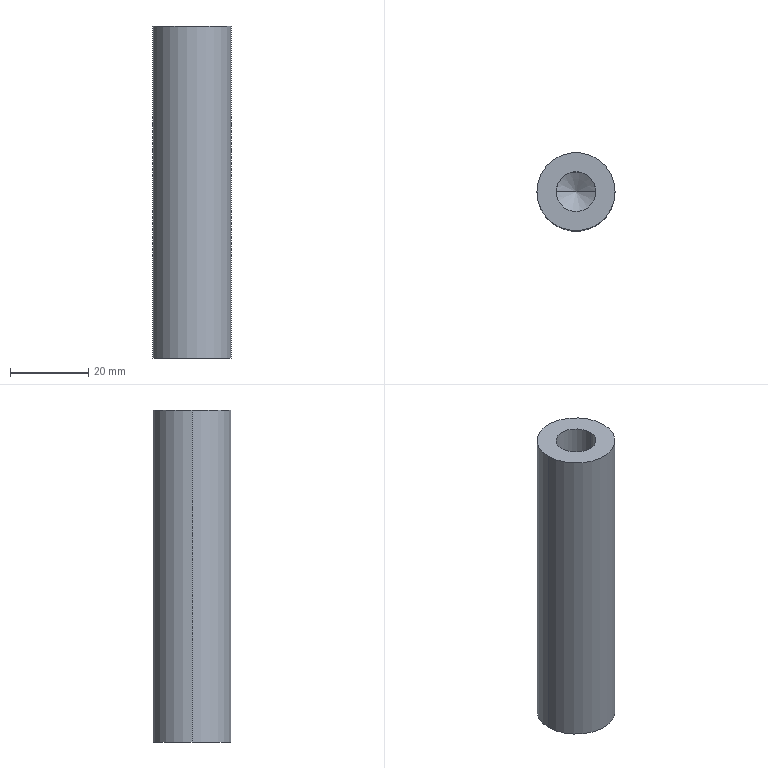Part | SolidWorks | features BaseBody 1 | 1 solid | 12 faces | box 20 x 20 x 85 mm | volume 21756 mm3 | cylinder 6 | cone 4 | plane 2 | commonest cylinder face diameters 10.2 x4 20 x2
STEP:
#1=CARTESIAN_POINT('',(105.,-44.517,369.481));
#2=VERTEX_POINT('',#1);
#3=CARTESIAN_POINT('',(125.,-44.517,369.481));
#4=VERTEX_POINT('',#3);
#5=CARTESIAN_POINT('',(115.,-44.517,369.481));
#6=DIRECTION('',(0.,0.,-1.));
#7=DIRECTION('',(-1.,0.,0.));
#8=AXIS2_PLACEMENT_3D('',#5,#6,#7);
#9=CIRCLE('',#8,10.);
#10=EDGE_CURVE('',#2,#4,#9,.T.);
#11=ORIENTED_EDGE('',*,*,#10,.T.);
#12=CARTESIAN_POINT('',(125.,-44.517,284.481));
#13=VERTEX_POINT('',#12);
#14=CARTESIAN_POINT('',(125.,-44.517,369.481));
#15=DIRECTION('',(0.,0.,-1.));
#16=VECTOR('',#15,1000.);
#17=LINE('',#14,#16);
#18=EDGE_CURVE('',#4,#13,#17,.T.);
#19=ORIENTED_EDGE('',*,*,#18,.T.);
#20=CARTESIAN_POINT('',(105.,-44.517,284.481));
#21=VERTEX_POINT('',#20);
#22=CARTESIAN_POINT('',(115.,-44.517,284.481));
#23=DIRECTION('',(0.,0.,1.));
#24=DIRECTION('',(-1.,0.,0.));
#25=AXIS2_PLACEMENT_3D('',#22,#23,#24);
#26=CIRCLE('',#25,10.);
#27=EDGE_CURVE('',#13,#21,#26,.T.);
#28=ORIENTED_EDGE('',*,*,#27,.T.);
#29=CARTESIAN_POINT('',(105.,-44.517,369.481));
#30=DIRECTION('',(0.,0.,-1.));
#31=VECTOR('',#30,1000.);
#32=LINE('',#29,#31);
#33=EDGE_CURVE('',#2,#21,#32,.T.);
#34=ORIENTED_EDGE('',*,*,#33,.F.);
#35=EDGE_LOOP('',(#11,#19,#28,#34));
#36=FACE_OUTER_BOUND('',#35,.T.);
#37=CARTESIAN_POINT('',(115.,-44.517,369.481));
#38=DIRECTION('',(0.,0.,-1.));
#39=DIRECTION('',(-1.,0.,0.));
#40=AXIS2_PLACEMENT_3D('',#37,#38,#39);
#41=CYLINDRICAL_SURFACE('',#40,10.);
#42=ADVANCED_FACE('',(#36),#41,.T.);
#43=CARTESIAN_POINT('',(120.1,-44.517,313.731));
#44=VERTEX_POINT('',#43);
#45=CARTESIAN_POINT('',(109.9,-44.517,313.731));
#46=VERTEX_POINT('',#45);
#47=CARTESIAN_POINT('',(115.,-44.517,313.731));
#48=DIRECTION('',(0.,0.,-1.));
#49=DIRECTION('',(-1.,0.,0.));
#50=AXIS2_PLACEMENT_3D('',#47,#48,#49);
#51=CIRCLE('',#50,5.1);
#52=EDGE_CURVE('',#44,#46,#51,.T.);
#53=ORIENTED_EDGE('',*,*,#52,.F.);
#54=CARTESIAN_POINT('',(120.1,-44.517,284.481));
#55=VERTEX_POINT('',#54);
#56=CARTESIAN_POINT('',(120.1,-44.517,284.481));
#57=DIRECTION('',(0.,0.,-1.));
#58=VECTOR('',#57,1000.);
#59=LINE('',#56,#58);
#60=EDGE_CURVE('',#44,#55,#59,.T.);
#61=ORIENTED_EDGE('',*,*,#60,.T.);
#62=CARTESIAN_POINT('',(109.9,-44.517,284.481));
#63=VERTEX_POINT('',#62);
#64=CARTESIAN_POINT('',(115.,-44.517,284.481));
#65=DIRECTION('',(0.,0.,-1.));
#66=DIRECTION('',(-1.,0.,0.));
#67=AXIS2_PLACEMENT_3D('',#64,#65,#66);
#68=CIRCLE('',#67,5.1);
#69=EDGE_CURVE('',#55,#63,#68,.T.);
#70=ORIENTED_EDGE('',*,*,#69,.T.);
#71=CARTESIAN_POINT('',(109.9,-44.517,284.481));
#72=DIRECTION('',(0.,0.,-1.));
#73=VECTOR('',#72,1000.);
#74=LINE('',#71,#73);
#75=EDGE_CURVE('',#46,#63,#74,.T.);
#76=ORIENTED_EDGE('',*,*,#75,.F.);
#77=EDGE_LOOP('',(#53,#61,#70,#76));
#78=FACE_OUTER_BOUND('',#77,.T.);
#79=CARTESIAN_POINT('',(115.,-44.517,284.481));
#80=DIRECTION('',(0.,0.,-1.));
#81=DIRECTION('',(-1.,0.,0.));
#82=AXIS2_PLACEMENT_3D('',#79,#80,#81);
#83=CYLINDRICAL_SURFACE('',#82,5.1);
#84=ADVANCED_FACE('',(#78),#83,.F.);
#85=CARTESIAN_POINT('',(109.9,-44.517,340.231));
#86=VERTEX_POINT('',#85);
#87=CARTESIAN_POINT('',(120.1,-44.517,340.231));
#88=VERTEX_POINT('',#87);
#89=CARTESIAN_POINT('',(115.,-44.517,340.231));
#90=DIRECTION('',(0.,0.,1.));
#91=DIRECTION('',(1.,0.,0.));
#92=AXIS2_PLACEMENT_3D('',#89,#90,#91);
#93=CIRCLE('',#92,5.1);
#94=EDGE_CURVE('',#86,#88,#93,.T.);
#95=ORIENTED_EDGE('',*,*,#94,.F.);
#96=CARTESIAN_POINT('',(109.9,-44.517,369.481));
#97=VERTEX_POINT('',#96);
#98=CARTESIAN_POINT('',(109.9,-44.517,369.481));
#99=DIRECTION('',(0.,0.,1.));
#100=VECTOR('',#99,1000.);
#101=LINE('',#98,#100);
#102=EDGE_CURVE('',#86,#97,#101,.T.);
#103=ORIENTED_EDGE('',*,*,#102,.T.);
#104=CARTESIAN_POINT('',(120.1,-44.517,369.481));
#105=VERTEX_POINT('',#104);
#106=CARTESIAN_POINT('',(115.,-44.517,369.481));
#107=DIRECTION('',(0.,0.,-1.));
#108=DIRECTION('',(1.,0.,0.));
#109=AXIS2_PLACEMENT_3D('',#106,#107,#108);
#110=CIRCLE('',#109,5.1);
#111=EDGE_CURVE('',#105,#97,#110,.T.);
#112=ORIENTED_EDGE('',*,*,#111,.F.);
#113=CARTESIAN_POINT('',(120.1,-44.517,369.481));
#114=DIRECTION('',(0.,0.,1.));
#115=VECTOR('',#114,1000.);
#116=LINE('',#113,#115);
#117=EDGE_CURVE('',#88,#105,#116,.T.);
#118=ORIENTED_EDGE('',*,*,#117,.F.);
#119=EDGE_LOOP('',(#95,#103,#112,#118));
#120=FACE_OUTER_BOUND('',#119,.T.);
#121=CARTESIAN_POINT('',(115.,-44.517,369.481));
#122=DIRECTION('',(0.,0.,1.));
#123=DIRECTION('',(1.,0.,0.));
#124=AXIS2_PLACEMENT_3D('',#121,#122,#123);
#125=CYLINDRICAL_SURFACE('',#124,5.1);
#126=ADVANCED_FACE('',(#120),#125,.F.);
#127=CARTESIAN_POINT('',(115.,-44.517,316.795));
#128=VERTEX_POINT('',#127);
#129=CARTESIAN_POINT('',(109.9,-44.517,313.731));
#130=DIRECTION('',(-0.8572,0.,-0.515));
#131=VECTOR('',#130,1000.);
#132=LINE('',#129,#131);
#133=EDGE_CURVE('',#128,#46,#132,.T.);
#134=ORIENTED_EDGE('',*,*,#133,.F.);
#135=CARTESIAN_POINT('',(120.1,-44.517,313.731));
#136=DIRECTION('',(0.8572,0.,-0.515));
#137=VECTOR('',#136,1000.);
#138=LINE('',#135,#137);
#139=EDGE_CURVE('',#128,#44,#138,.T.);
#140=ORIENTED_EDGE('',*,*,#139,.T.);
#141=ORIENTED_EDGE('',*,*,#52,.T.);
#142=EDGE_LOOP('',(#134,#140,#141));
#143=FACE_OUTER_BOUND('',#142,.T.);
#144=CARTESIAN_POINT('',(115.,-44.517,313.731));
#145=DIRECTION('',(0.,0.,-1.));
#146=DIRECTION('',(-1.,0.,0.));
#147=AXIS2_PLACEMENT_3D('',#144,#145,#146);
#148=CONICAL_SURFACE('',#147,5.1,1.03);
#149=ADVANCED_FACE('',(#143),#148,.F.);
#150=CARTESIAN_POINT('',(115.,-44.517,337.167));
#151=VERTEX_POINT('',#150);
#152=CARTESIAN_POINT('',(120.1,-44.517,340.231));
#153=DIRECTION('',(0.8572,0.,0.515));
#154=VECTOR('',#153,1000.);
#155=LINE('',#152,#154);
#156=EDGE_CURVE('',#151,#88,#155,.T.);
#157=ORIENTED_EDGE('',*,*,#156,.F.);
#158=CARTESIAN_POINT('',(109.9,-44.517,340.231));
#159=DIRECTION('',(-0.8572,0.,0.515));
#160=VECTOR('',#159,1000.);
#161=LINE('',#158,#160);
#162=EDGE_CURVE('',#151,#86,#161,.T.);
#163=ORIENTED_EDGE('',*,*,#162,.T.);
#164=ORIENTED_EDGE('',*,*,#94,.T.);
#165=EDGE_LOOP('',(#157,#163,#164));
#166=FACE_OUTER_BOUND('',#165,.T.);
#167=CARTESIAN_POINT('',(115.,-44.517,340.231));
#168=DIRECTION('',(0.,0.,1.));
#169=DIRECTION('',(1.,0.,0.));
#170=AXIS2_PLACEMENT_3D('',#167,#168,#169);
#171=CONICAL_SURFACE('',#170,5.1,1.03);
#172=ADVANCED_FACE('',(#166),#171,.F.);
#173=ORIENTED_EDGE('',*,*,#18,.F.);
#174=CARTESIAN_POINT('',(115.,-44.517,369.481));
#175=DIRECTION('',(0.,0.,-1.));
#176=DIRECTION('',(-1.,0.,0.));
#177=AXIS2_PLACEMENT_3D('',#174,#175,#176);
#178=CIRCLE('',#177,10.);
#179=EDGE_CURVE('',#4,#2,#178,.T.);
#180=ORIENTED_EDGE('',*,*,#179,.T.);
#181=ORIENTED_EDGE('',*,*,#33,.T.);
#182=CARTESIAN_POINT('',(115.,-44.517,284.481));
#183=DIRECTION('',(0.,0.,1.));
#184=DIRECTION('',(-1.,0.,0.));
#185=AXIS2_PLACEMENT_3D('',#182,#183,#184);
#186=CIRCLE('',#185,10.);
#187=EDGE_CURVE('',#21,#13,#186,.T.);
#188=ORIENTED_EDGE('',*,*,#187,.T.);
#189=EDGE_LOOP('',(#173,#180,#181,#188));
#190=FACE_OUTER_BOUND('',#189,.T.);
#191=CARTESIAN_POINT('',(115.,-44.517,369.481));
#192=DIRECTION('',(0.,0.,-1.));
#193=DIRECTION('',(-1.,0.,0.));
#194=AXIS2_PLACEMENT_3D('',#191,#192,#193);
#195=CYLINDRICAL_SURFACE('',#194,10.);
#196=ADVANCED_FACE('',(#190),#195,.T.);
#197=ORIENTED_EDGE('',*,*,#187,.F.);
#198=ORIENTED_EDGE('',*,*,#27,.F.);
#199=EDGE_LOOP('',(#197,#198));
#200=FACE_OUTER_BOUND('',#199,.T.);
#201=CARTESIAN_POINT('',(115.,-44.517,284.481));
#202=DIRECTION('',(0.,0.,-1.));
#203=DIRECTION('',(-1.,0.,0.));
#204=AXIS2_PLACEMENT_3D('',#201,#202,#203);
#205=CIRCLE('',#204,5.1);
#206=EDGE_CURVE('',#63,#55,#205,.T.);
#207=ORIENTED_EDGE('',*,*,#206,.F.);
#208=ORIENTED_EDGE('',*,*,#69,.F.);
#209=EDGE_LOOP('',(#207,#208));
#210=FACE_BOUND('',#209,.T.);
#211=CARTESIAN_POINT('',(115.,-44.517,284.481));
#212=DIRECTION('',(0.,0.,1.));
#213=DIRECTION('',(1.,0.,0.));
#214=AXIS2_PLACEMENT_3D('',#211,#212,#213);
#215=PLANE('',#214);
#216=ADVANCED_FACE('',(#200,#210),#215,.F.);
#217=ORIENTED_EDGE('',*,*,#10,.F.);
#218=ORIENTED_EDGE('',*,*,#179,.F.);
#219=EDGE_LOOP('',(#217,#218));
#220=FACE_OUTER_BOUND('',#219,.T.);
#221=ORIENTED_EDGE('',*,*,#111,.T.);
#222=CARTESIAN_POINT('',(115.,-44.517,369.481));
#223=DIRECTION('',(0.,0.,-1.));
#224=DIRECTION('',(1.,0.,0.));
#225=AXIS2_PLACEMENT_3D('',#222,#223,#224);
#226=CIRCLE('',#225,5.1);
#227=EDGE_CURVE('',#97,#105,#226,.T.);
#228=ORIENTED_EDGE('',*,*,#227,.T.);
#229=EDGE_LOOP('',(#221,#228));
#230=FACE_BOUND('',#229,.T.);
#231=CARTESIAN_POINT('',(115.,-44.517,369.481));
#232=DIRECTION('',(0.,0.,1.));
#233=DIRECTION('',(1.,0.,0.));
#234=AXIS2_PLACEMENT_3D('',#231,#232,#233);
#235=PLANE('',#234);
#236=ADVANCED_FACE('',(#220,#230),#235,.T.);
#237=ORIENTED_EDGE('',*,*,#60,.F.);
#238=CARTESIAN_POINT('',(115.,-44.517,313.731));
#239=DIRECTION('',(0.,0.,-1.));
#240=DIRECTION('',(-1.,0.,0.));
#241=AXIS2_PLACEMENT_3D('',#238,#239,#240);
#242=CIRCLE('',#241,5.1);
#243=EDGE_CURVE('',#46,#44,#242,.T.);
#244=ORIENTED_EDGE('',*,*,#243,.F.);
#245=ORIENTED_EDGE('',*,*,#75,.T.);
#246=ORIENTED_EDGE('',*,*,#206,.T.);
#247=EDGE_LOOP('',(#237,#244,#245,#246));
#248=FACE_OUTER_BOUND('',#247,.T.);
#249=CARTESIAN_POINT('',(115.,-44.517,284.481));
#250=DIRECTION('',(0.,0.,-1.));
#251=DIRECTION('',(-1.,0.,0.));
#252=AXIS2_PLACEMENT_3D('',#249,#250,#251);
#253=CYLINDRICAL_SURFACE('',#252,5.1);
#254=ADVANCED_FACE('',(#248),#253,.F.);
#255=ORIENTED_EDGE('',*,*,#102,.F.);
#256=CARTESIAN_POINT('',(115.,-44.517,340.231));
#257=DIRECTION('',(0.,0.,1.));
#258=DIRECTION('',(1.,0.,0.));
#259=AXIS2_PLACEMENT_3D('',#256,#257,#258);
#260=CIRCLE('',#259,5.1);
#261=EDGE_CURVE('',#88,#86,#260,.T.);
#262=ORIENTED_EDGE('',*,*,#261,.F.);
#263=ORIENTED_EDGE('',*,*,#117,.T.);
#264=ORIENTED_EDGE('',*,*,#227,.F.);
#265=EDGE_LOOP('',(#255,#262,#263,#264));
#266=FACE_OUTER_BOUND('',#265,.T.);
#267=CARTESIAN_POINT('',(115.,-44.517,369.481));
#268=DIRECTION('',(0.,0.,1.));
#269=DIRECTION('',(1.,0.,0.));
#270=AXIS2_PLACEMENT_3D('',#267,#268,#269);
#271=CYLINDRICAL_SURFACE('',#270,5.1);
#272=ADVANCED_FACE('',(#266),#271,.F.);
#273=ORIENTED_EDGE('',*,*,#139,.F.);
#274=ORIENTED_EDGE('',*,*,#133,.T.);
#275=ORIENTED_EDGE('',*,*,#243,.T.);
#276=EDGE_LOOP('',(#273,#274,#275));
#277=FACE_OUTER_BOUND('',#276,.T.);
#278=CARTESIAN_POINT('',(115.,-44.517,313.731));
#279=DIRECTION('',(0.,0.,-1.));
#280=DIRECTION('',(-1.,0.,0.));
#281=AXIS2_PLACEMENT_3D('',#278,#279,#280);
#282=CONICAL_SURFACE('',#281,5.1,1.03);
#283=ADVANCED_FACE('',(#277),#282,.F.);
#284=ORIENTED_EDGE('',*,*,#162,.F.);
#285=ORIENTED_EDGE('',*,*,#156,.T.);
#286=ORIENTED_EDGE('',*,*,#261,.T.);
#287=EDGE_LOOP('',(#284,#285,#286));
#288=FACE_OUTER_BOUND('',#287,.T.);
#289=CARTESIAN_POINT('',(115.,-44.517,340.231));
#290=DIRECTION('',(0.,0.,1.));
#291=DIRECTION('',(1.,0.,0.));
#292=AXIS2_PLACEMENT_3D('',#289,#290,#291);
#293=CONICAL_SURFACE('',#292,5.1,1.03);
#294=ADVANCED_FACE('',(#288),#293,.F.);
#295=CLOSED_SHELL('',(#42,#84,#126,#149,#172,#196,#216,#236,#254,#272,#283,#294));
#296=MANIFOLD_SOLID_BREP('',#295);
#297=CARTESIAN_POINT('',(0.,0.,0.));
#298=DIRECTION('',(0.,0.,1.));
#299=DIRECTION('',(1.,0.,0.));
#300=AXIS2_PLACEMENT_3D('',#297,#298,#299);
#301=(LENGTH_UNIT()NAMED_UNIT(*)SI_UNIT(.MILLI.,.METRE.));
#302=UNCERTAINTY_MEASURE_WITH_UNIT(LENGTH_MEASURE(0.00001),#301,'','');
#303=(NAMED_UNIT(*)PLANE_ANGLE_UNIT()SI_UNIT($,.RADIAN.));
#304=(NAMED_UNIT(*)SI_UNIT($,.STERADIAN.)SOLID_ANGLE_UNIT());
#305=(GEOMETRIC_REPRESENTATION_CONTEXT(3)GLOBAL_UNCERTAINTY_ASSIGNED_CONTEXT((#302))GLOBAL_UNIT_ASSIGNED_CONTEXT((#301,#303,#304))REPRESENTATION_CONTEXT('',''));
#306=ADVANCED_BREP_SHAPE_REPRESENTATION('',(#296,#300),#305);